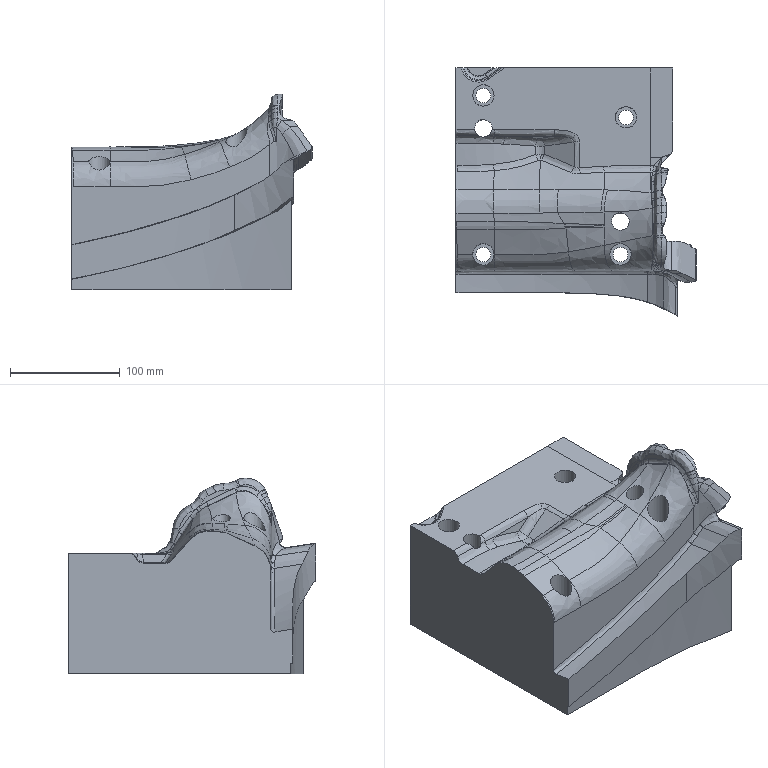Part | NX | features solid 2 | 1 solid | 189 faces | box 218.876 x 226.12 x 178.566 mm | volume 4388760 mm3 | spline 166 | plane 13 | cylinder 10 | commonest cylinder face diameters 13.5 x4 19.5 x4 16 x2